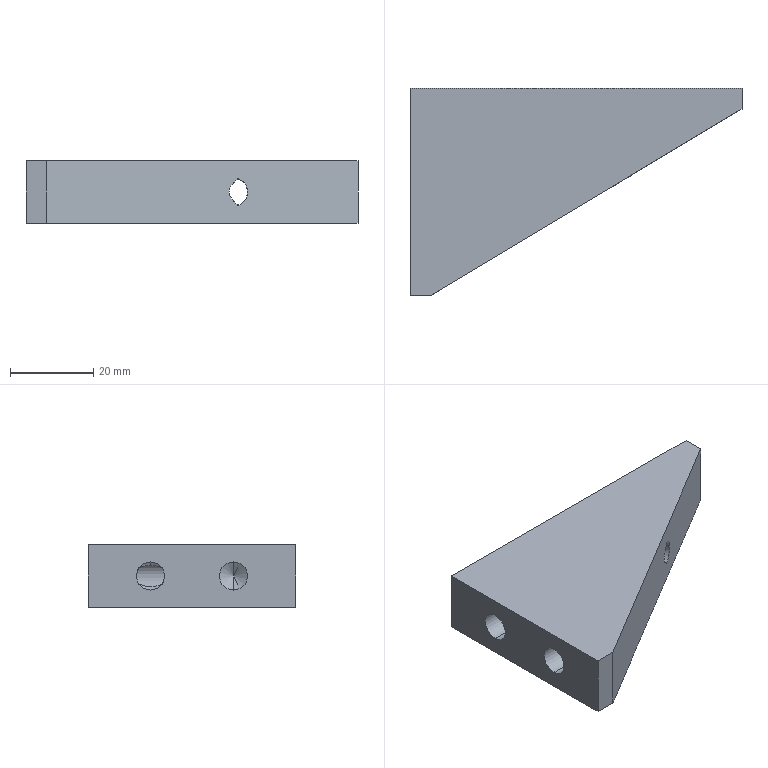Part | SolidWorks | features HoleWzd 2, Extrusion 1 | 1 solid | 25 faces | box 80 x 50 x 15 mm | volume 31407 mm3 | cone 10 | cylinder 8 | plane 7 | commonest cylinder face diameters 6.8 x8
STEP:
#1=CARTESIAN_POINT('',(22.757,35.,10.056));
#2=VERTEX_POINT('',#1);
#3=CARTESIAN_POINT('',(22.25,37.75,9.499));
#4=VERTEX_POINT('',#3);
#5=CARTESIAN_POINT('',(22.757,35.,10.056));
#6=CARTESIAN_POINT('',(22.757,35.242,10.056));
#7=CARTESIAN_POINT('',(22.744,35.483,10.044));
#8=CARTESIAN_POINT('',(22.692,35.956,9.997));
#9=CARTESIAN_POINT('',(22.655,36.19,9.963));
#10=CARTESIAN_POINT('',(22.562,36.651,9.871));
#11=CARTESIAN_POINT('',(22.506,36.88,9.813));
#12=CARTESIAN_POINT('',(22.384,37.325,9.674));
#13=CARTESIAN_POINT('',(22.318,37.541,9.594));
#14=CARTESIAN_POINT('',(22.25,37.75,9.499));
#15=B_SPLINE_CURVE_WITH_KNOTS('',3,(#5,#6,#7,#8,#9,#10,#11,#12,#13,#14),.UNSPECIFIED.,.F.,.F.,(4,2,2,2,4),(0.003573,0.004291,0.005009,0.005727,0.006445),.UNSPECIFIED.);
#16=EDGE_CURVE('',#2,#4,#15,.T.);
#17=ORIENTED_EDGE('',*,*,#16,.F.);
#18=CARTESIAN_POINT('',(22.25,35.,10.9));
#19=VERTEX_POINT('',#18);
#20=CARTESIAN_POINT('',(22.25,35.,10.9));
#21=DIRECTION('',(-0.515,0.,0.8572));
#22=VECTOR('',#21,1000.);
#23=LINE('',#20,#22);
#24=EDGE_CURVE('',#2,#19,#23,.T.);
#25=ORIENTED_EDGE('',*,*,#24,.T.);
#26=CARTESIAN_POINT('',(22.25,35.,7.5));
#27=DIRECTION('',(-1.,0.,0.));
#28=DIRECTION('',(0.,0.,1.));
#29=AXIS2_PLACEMENT_3D('',#26,#27,#28);
#30=CIRCLE('',#29,3.4);
#31=EDGE_CURVE('',#19,#4,#30,.T.);
#32=ORIENTED_EDGE('',*,*,#31,.T.);
#33=EDGE_LOOP('',(#17,#25,#32));
#34=FACE_OUTER_BOUND('',#33,.T.);
#35=CARTESIAN_POINT('',(22.25,35.,7.5));
#36=DIRECTION('',(-1.,0.,0.));
#37=DIRECTION('',(0.,0.,1.));
#38=AXIS2_PLACEMENT_3D('',#35,#36,#37);
#39=CONICAL_SURFACE('',#38,3.4,1.03);
#40=ADVANCED_FACE('',(#34),#39,.F.);
#41=CARTESIAN_POINT('',(22.25,35.,4.1));
#42=VERTEX_POINT('',#41);
#43=CARTESIAN_POINT('',(22.25,32.25,5.501));
#44=VERTEX_POINT('',#43);
#45=CARTESIAN_POINT('',(22.25,35.,7.5));
#46=DIRECTION('',(-1.,0.,0.));
#47=DIRECTION('',(0.,0.,1.));
#48=AXIS2_PLACEMENT_3D('',#45,#46,#47);
#49=CIRCLE('',#48,3.4);
#50=EDGE_CURVE('',#42,#44,#49,.T.);
#51=ORIENTED_EDGE('',*,*,#50,.F.);
#52=CARTESIAN_POINT('',(0.,35.,4.1));
#53=VERTEX_POINT('',#52);
#54=CARTESIAN_POINT('',(0.,35.,4.1));
#55=DIRECTION('',(-1.,0.,0.));
#56=VECTOR('',#55,1000.);
#57=LINE('',#54,#56);
#58=EDGE_CURVE('',#42,#53,#57,.T.);
#59=ORIENTED_EDGE('',*,*,#58,.T.);
#60=CARTESIAN_POINT('',(0.,35.,10.9));
#61=VERTEX_POINT('',#60);
#62=CARTESIAN_POINT('',(0.,35.,7.5));
#63=DIRECTION('',(-1.,0.,0.));
#64=DIRECTION('',(0.,0.,1.));
#65=AXIS2_PLACEMENT_3D('',#62,#63,#64);
#66=CIRCLE('',#65,3.4);
#67=EDGE_CURVE('',#53,#61,#66,.T.);
#68=ORIENTED_EDGE('',*,*,#67,.T.);
#69=CARTESIAN_POINT('',(0.,35.,10.9));
#70=DIRECTION('',(-1.,0.,0.));
#71=VECTOR('',#70,1000.);
#72=LINE('',#69,#71);
#73=EDGE_CURVE('',#19,#61,#72,.T.);
#74=ORIENTED_EDGE('',*,*,#73,.F.);
#75=CARTESIAN_POINT('',(22.25,32.25,9.499));
#76=VERTEX_POINT('',#75);
#77=CARTESIAN_POINT('',(22.25,35.,7.5));
#78=DIRECTION('',(-1.,0.,0.));
#79=DIRECTION('',(0.,0.,1.));
#80=AXIS2_PLACEMENT_3D('',#77,#78,#79);
#81=CIRCLE('',#80,3.4);
#82=EDGE_CURVE('',#76,#19,#81,.T.);
#83=ORIENTED_EDGE('',*,*,#82,.F.);
#84=CARTESIAN_POINT('',(22.25,32.25,5.501));
#85=CARTESIAN_POINT('',(21.352,31.352,6.736));
#86=CARTESIAN_POINT('',(21.352,31.352,8.264));
#87=CARTESIAN_POINT('',(22.25,32.25,9.499));
#88=(BOUNDED_CURVE()B_SPLINE_CURVE(3,(#84,#85,#86,#87),.UNSPECIFIED.,.F.,.F.)B_SPLINE_CURVE_WITH_KNOTS((4,4),(2.513,3.77),.UNSPECIFIED.)CURVE()GEOMETRIC_REPRESENTATION_ITEM()RATIONAL_B_SPLINE_CURVE((1.,0.8725,0.8725,1.))REPRESENTATION_ITEM(''));
#89=EDGE_CURVE('',#44,#76,#88,.T.);
#90=ORIENTED_EDGE('',*,*,#89,.F.);
#91=EDGE_LOOP('',(#51,#59,#68,#74,#83,#90));
#92=FACE_OUTER_BOUND('',#91,.T.);
#93=CARTESIAN_POINT('',(0.,35.,7.5));
#94=DIRECTION('',(-1.,0.,0.));
#95=DIRECTION('',(0.,0.,1.));
#96=AXIS2_PLACEMENT_3D('',#93,#94,#95);
#97=CYLINDRICAL_SURFACE('',#96,3.4);
#98=ADVANCED_FACE('',(#92),#97,.F.);
#99=CARTESIAN_POINT('',(22.25,15.,4.1));
#100=VERTEX_POINT('',#99);
#101=CARTESIAN_POINT('',(22.25,15.,10.9));
#102=VERTEX_POINT('',#101);
#103=CARTESIAN_POINT('',(22.25,15.,7.5));
#104=DIRECTION('',(-1.,0.,0.));
#105=DIRECTION('',(0.,0.,1.));
#106=AXIS2_PLACEMENT_3D('',#103,#104,#105);
#107=CIRCLE('',#106,3.4);
#108=EDGE_CURVE('',#100,#102,#107,.T.);
#109=ORIENTED_EDGE('',*,*,#108,.F.);
#110=CARTESIAN_POINT('',(0.,15.,4.1));
#111=VERTEX_POINT('',#110);
#112=CARTESIAN_POINT('',(0.,15.,4.1));
#113=DIRECTION('',(-1.,0.,0.));
#114=VECTOR('',#113,1000.);
#115=LINE('',#112,#114);
#116=EDGE_CURVE('',#100,#111,#115,.T.);
#117=ORIENTED_EDGE('',*,*,#116,.T.);
#118=CARTESIAN_POINT('',(0.,15.,10.9));
#119=VERTEX_POINT('',#118);
#120=CARTESIAN_POINT('',(0.,15.,7.5));
#121=DIRECTION('',(-1.,0.,0.));
#122=DIRECTION('',(0.,0.,1.));
#123=AXIS2_PLACEMENT_3D('',#120,#121,#122);
#124=CIRCLE('',#123,3.4);
#125=EDGE_CURVE('',#111,#119,#124,.T.);
#126=ORIENTED_EDGE('',*,*,#125,.T.);
#127=CARTESIAN_POINT('',(0.,15.,10.9));
#128=DIRECTION('',(-1.,0.,0.));
#129=VECTOR('',#128,1000.);
#130=LINE('',#127,#129);
#131=EDGE_CURVE('',#102,#119,#130,.T.);
#132=ORIENTED_EDGE('',*,*,#131,.F.);
#133=EDGE_LOOP('',(#109,#117,#126,#132));
#134=FACE_OUTER_BOUND('',#133,.T.);
#135=CARTESIAN_POINT('',(0.,15.,7.5));
#136=DIRECTION('',(-1.,0.,0.));
#137=DIRECTION('',(0.,0.,1.));
#138=AXIS2_PLACEMENT_3D('',#135,#136,#137);
#139=CYLINDRICAL_SURFACE('',#138,3.4);
#140=ADVANCED_FACE('',(#134),#139,.F.);
#141=CARTESIAN_POINT('',(24.293,15.,7.5));
#142=VERTEX_POINT('',#141);
#143=CARTESIAN_POINT('',(22.25,15.,10.9));
#144=DIRECTION('',(-0.515,0.,0.8572));
#145=VECTOR('',#144,1000.);
#146=LINE('',#143,#145);
#147=EDGE_CURVE('',#142,#102,#146,.T.);
#148=ORIENTED_EDGE('',*,*,#147,.F.);
#149=CARTESIAN_POINT('',(22.25,15.,4.1));
#150=DIRECTION('',(-0.515,0.,-0.8572));
#151=VECTOR('',#150,1000.);
#152=LINE('',#149,#151);
#153=EDGE_CURVE('',#142,#100,#152,.T.);
#154=ORIENTED_EDGE('',*,*,#153,.T.);
#155=ORIENTED_EDGE('',*,*,#108,.T.);
#156=EDGE_LOOP('',(#148,#154,#155));
#157=FACE_OUTER_BOUND('',#156,.T.);
#158=CARTESIAN_POINT('',(22.25,15.,7.5));
#159=DIRECTION('',(-1.,0.,0.));
#160=DIRECTION('',(0.,0.,1.));
#161=AXIS2_PLACEMENT_3D('',#158,#159,#160);
#162=CONICAL_SURFACE('',#161,3.4,1.03);
#163=ADVANCED_FACE('',(#157),#162,.F.);
#164=CARTESIAN_POINT('',(22.25,37.75,5.501));
#165=VERTEX_POINT('',#164);
#166=CARTESIAN_POINT('',(22.25,37.75,9.499));
#167=CARTESIAN_POINT('',(21.352,38.648,8.264));
#168=CARTESIAN_POINT('',(21.352,38.648,6.736));
#169=CARTESIAN_POINT('',(22.25,37.75,5.501));
#170=(BOUNDED_CURVE()B_SPLINE_CURVE(3,(#166,#167,#168,#169),.UNSPECIFIED.,.F.,.F.)B_SPLINE_CURVE_WITH_KNOTS((4,4),(5.655,6.912),.UNSPECIFIED.)CURVE()GEOMETRIC_REPRESENTATION_ITEM()RATIONAL_B_SPLINE_CURVE((1.,0.8725,0.8725,1.))REPRESENTATION_ITEM(''));
#171=EDGE_CURVE('',#4,#165,#170,.T.);
#172=ORIENTED_EDGE('',*,*,#171,.T.);
#173=CARTESIAN_POINT('',(22.25,37.75,5.501));
#174=CARTESIAN_POINT('',(22.318,37.541,5.406));
#175=CARTESIAN_POINT('',(22.384,37.325,5.326));
#176=CARTESIAN_POINT('',(22.506,36.881,5.187));
#177=CARTESIAN_POINT('',(22.562,36.651,5.129));
#178=CARTESIAN_POINT('',(22.702,35.958,4.991));
#179=CARTESIAN_POINT('',(22.757,35.486,4.945));
#180=CARTESIAN_POINT('',(22.757,34.76,4.944));
#181=CARTESIAN_POINT('',(22.744,34.519,4.956));
#182=CARTESIAN_POINT('',(22.693,34.045,5.003));
#183=CARTESIAN_POINT('',(22.655,33.812,5.037));
#184=CARTESIAN_POINT('',(22.562,33.35,5.129));
#185=CARTESIAN_POINT('',(22.506,33.12,5.187));
#186=CARTESIAN_POINT('',(22.385,32.676,5.326));
#187=CARTESIAN_POINT('',(22.319,32.46,5.406));
#188=CARTESIAN_POINT('',(22.25,32.25,5.501));
#189=B_SPLINE_CURVE_WITH_KNOTS('',3,(#173,#174,#175,#176,#177,#178,#179,#180,#181,#182,#183,#184,#185,#186,#187,#188),.UNSPECIFIED.,.F.,.F.,(4,2,2,2,2,2,2,4),(0.0006976,0.001416,0.002134,0.003571,0.004289,0.005008,0.005726,0.006445),.UNSPECIFIED.);
#190=EDGE_CURVE('',#165,#44,#189,.T.);
#191=ORIENTED_EDGE('',*,*,#190,.T.);
#192=ORIENTED_EDGE('',*,*,#89,.T.);
#193=CARTESIAN_POINT('',(22.25,32.25,9.499));
#194=CARTESIAN_POINT('',(22.319,32.46,9.594));
#195=CARTESIAN_POINT('',(22.385,32.675,9.674));
#196=CARTESIAN_POINT('',(22.506,33.12,9.813));
#197=CARTESIAN_POINT('',(22.562,33.35,9.871));
#198=CARTESIAN_POINT('',(22.702,34.043,10.009));
#199=CARTESIAN_POINT('',(22.757,34.515,10.056));
#200=CARTESIAN_POINT('',(22.757,35.,10.056));
#201=B_SPLINE_CURVE_WITH_KNOTS('',3,(#193,#194,#195,#196,#197,#198,#199,#200),.UNSPECIFIED.,.F.,.F.,(4,2,2,4),(0.0006976,0.001416,0.002135,0.003573),.UNSPECIFIED.);
#202=EDGE_CURVE('',#76,#2,#201,.T.);
#203=ORIENTED_EDGE('',*,*,#202,.T.);
#204=ORIENTED_EDGE('',*,*,#16,.T.);
#205=EDGE_LOOP('',(#172,#191,#192,#203,#204));
#206=FACE_BOUND('',#205,.T.);
#207=CARTESIAN_POINT('',(25.,27.75,4.1));
#208=VERTEX_POINT('',#207);
#209=CARTESIAN_POINT('',(25.,27.75,10.9));
#210=VERTEX_POINT('',#209);
#211=CARTESIAN_POINT('',(25.,27.75,7.5));
#212=DIRECTION('',(0.,1.,0.));
#213=DIRECTION('',(0.,0.,1.));
#214=AXIS2_PLACEMENT_3D('',#211,#212,#213);
#215=CIRCLE('',#214,3.4);
#216=EDGE_CURVE('',#208,#210,#215,.T.);
#217=ORIENTED_EDGE('',*,*,#216,.F.);
#218=CARTESIAN_POINT('',(25.,50.,4.1));
#219=VERTEX_POINT('',#218);
#220=CARTESIAN_POINT('',(25.,50.,4.1));
#221=DIRECTION('',(0.,1.,0.));
#222=VECTOR('',#221,1000.);
#223=LINE('',#220,#222);
#224=EDGE_CURVE('',#208,#219,#223,.T.);
#225=ORIENTED_EDGE('',*,*,#224,.T.);
#226=CARTESIAN_POINT('',(25.,50.,10.9));
#227=VERTEX_POINT('',#226);
#228=CARTESIAN_POINT('',(25.,50.,7.5));
#229=DIRECTION('',(0.,1.,0.));
#230=DIRECTION('',(0.,0.,1.));
#231=AXIS2_PLACEMENT_3D('',#228,#229,#230);
#232=CIRCLE('',#231,3.4);
#233=EDGE_CURVE('',#219,#227,#232,.T.);
#234=ORIENTED_EDGE('',*,*,#233,.T.);
#235=CARTESIAN_POINT('',(25.,50.,10.9));
#236=DIRECTION('',(0.,1.,0.));
#237=VECTOR('',#236,1000.);
#238=LINE('',#235,#237);
#239=EDGE_CURVE('',#210,#227,#238,.T.);
#240=ORIENTED_EDGE('',*,*,#239,.F.);
#241=EDGE_LOOP('',(#217,#225,#234,#240));
#242=FACE_OUTER_BOUND('',#241,.T.);
#243=CARTESIAN_POINT('',(25.,50.,7.5));
#244=DIRECTION('',(0.,1.,0.));
#245=DIRECTION('',(0.,0.,1.));
#246=AXIS2_PLACEMENT_3D('',#243,#244,#245);
#247=CYLINDRICAL_SURFACE('',#246,3.4);
#248=ADVANCED_FACE('',(#206,#242),#247,.F.);
#249=CARTESIAN_POINT('',(25.,25.707,7.5));
#250=VERTEX_POINT('',#249);
#251=CARTESIAN_POINT('',(25.,27.75,10.9));
#252=DIRECTION('',(0.,0.515,0.8572));
#253=VECTOR('',#252,1000.);
#254=LINE('',#251,#253);
#255=EDGE_CURVE('',#250,#210,#254,.T.);
#256=ORIENTED_EDGE('',*,*,#255,.F.);
#257=CARTESIAN_POINT('',(25.,27.75,4.1));
#258=DIRECTION('',(0.,0.515,-0.8572));
#259=VECTOR('',#258,1000.);
#260=LINE('',#257,#259);
#261=EDGE_CURVE('',#250,#208,#260,.T.);
#262=ORIENTED_EDGE('',*,*,#261,.T.);
#263=ORIENTED_EDGE('',*,*,#216,.T.);
#264=EDGE_LOOP('',(#256,#262,#263));
#265=FACE_OUTER_BOUND('',#264,.T.);
#266=CARTESIAN_POINT('',(25.,27.75,7.5));
#267=DIRECTION('',(0.,1.,0.));
#268=DIRECTION('',(0.,0.,1.));
#269=AXIS2_PLACEMENT_3D('',#266,#267,#268);
#270=CONICAL_SURFACE('',#269,3.4,1.03);
#271=ADVANCED_FACE('',(#265),#270,.F.);
#272=CARTESIAN_POINT('',(50.,27.,5.348));
#273=VERTEX_POINT('',#272);
#274=CARTESIAN_POINT('',(50.,27.,9.652));
#275=VERTEX_POINT('',#274);
#276=CARTESIAN_POINT('',(50.,27.,5.348));
#277=CARTESIAN_POINT('',(48.564,26.138,6.782));
#278=CARTESIAN_POINT('',(48.564,26.138,8.218));
#279=CARTESIAN_POINT('',(50.,27.,9.652));
#280=(BOUNDED_CURVE()B_SPLINE_CURVE(3,(#276,#277,#278,#279),.UNSPECIFIED.,.F.,.F.)B_SPLINE_CURVE_WITH_KNOTS((4,4),(3.088,3.195),.UNSPECIFIED.)CURVE()GEOMETRIC_REPRESENTATION_ITEM()RATIONAL_B_SPLINE_CURVE((1.,0.999,0.999,1.))REPRESENTATION_ITEM(''));
#281=EDGE_CURVE('',#273,#275,#280,.T.);
#282=ORIENTED_EDGE('',*,*,#281,.F.);
#283=CARTESIAN_POINT('',(50.,27.75,4.1));
#284=VERTEX_POINT('',#283);
#285=CARTESIAN_POINT('',(50.,27.75,4.1));
#286=DIRECTION('',(0.,0.515,-0.8572));
#287=VECTOR('',#286,1000.);
#288=LINE('',#285,#287);
#289=EDGE_CURVE('',#273,#284,#288,.T.);
#290=ORIENTED_EDGE('',*,*,#289,.T.);
#291=CARTESIAN_POINT('',(50.,27.75,10.9));
#292=VERTEX_POINT('',#291);
#293=CARTESIAN_POINT('',(50.,27.75,7.5));
#294=DIRECTION('',(0.,1.,0.));
#295=DIRECTION('',(0.,0.,1.));
#296=AXIS2_PLACEMENT_3D('',#293,#294,#295);
#297=CIRCLE('',#296,3.4);
#298=EDGE_CURVE('',#284,#292,#297,.T.);
#299=ORIENTED_EDGE('',*,*,#298,.T.);
#300=CARTESIAN_POINT('',(50.,27.75,10.9));
#301=DIRECTION('',(0.,0.515,0.8572));
#302=VECTOR('',#301,1000.);
#303=LINE('',#300,#302);
#304=EDGE_CURVE('',#275,#292,#303,.T.);
#305=ORIENTED_EDGE('',*,*,#304,.F.);
#306=EDGE_LOOP('',(#282,#290,#299,#305));
#307=FACE_OUTER_BOUND('',#306,.T.);
#308=CARTESIAN_POINT('',(50.,27.75,7.5));
#309=DIRECTION('',(0.,1.,0.));
#310=DIRECTION('',(0.,0.,1.));
#311=AXIS2_PLACEMENT_3D('',#308,#309,#310);
#312=CONICAL_SURFACE('',#311,3.4,1.03);
#313=ADVANCED_FACE('',(#307),#312,.F.);
#314=CARTESIAN_POINT('',(51.25,27.75,10.662));
#315=VERTEX_POINT('',#314);
#316=CARTESIAN_POINT('',(50.,27.,9.652));
#317=CARTESIAN_POINT('',(50.337,27.202,9.989));
#318=CARTESIAN_POINT('',(50.754,27.452,10.325));
#319=CARTESIAN_POINT('',(51.25,27.75,10.662));
#320=(BOUNDED_CURVE()B_SPLINE_CURVE(3,(#316,#317,#318,#319),.UNSPECIFIED.,.F.,.F.)B_SPLINE_CURVE_WITH_KNOTS((4,4),(3.195,3.22),.UNSPECIFIED.)CURVE()GEOMETRIC_REPRESENTATION_ITEM()RATIONAL_B_SPLINE_CURVE((1.,0.9999,0.9999,1.))REPRESENTATION_ITEM(''));
#321=EDGE_CURVE('',#275,#315,#320,.T.);
#322=ORIENTED_EDGE('',*,*,#321,.F.);
#323=ORIENTED_EDGE('',*,*,#304,.T.);
#324=CARTESIAN_POINT('',(50.,27.75,7.5));
#325=DIRECTION('',(0.,1.,0.));
#326=DIRECTION('',(0.,0.,1.));
#327=AXIS2_PLACEMENT_3D('',#324,#325,#326);
#328=CIRCLE('',#327,3.4);
#329=EDGE_CURVE('',#292,#315,#328,.T.);
#330=ORIENTED_EDGE('',*,*,#329,.T.);
#331=EDGE_LOOP('',(#322,#323,#330));
#332=FACE_OUTER_BOUND('',#331,.T.);
#333=CARTESIAN_POINT('',(50.,27.75,7.5));
#334=DIRECTION('',(0.,1.,0.));
#335=DIRECTION('',(0.,0.,1.));
#336=AXIS2_PLACEMENT_3D('',#333,#334,#335);
#337=CONICAL_SURFACE('',#336,3.4,1.03);
#338=ADVANCED_FACE('',(#332),#337,.F.);
#339=ORIENTED_EDGE('',*,*,#298,.F.);
#340=CARTESIAN_POINT('',(50.,50.,4.1));
#341=VERTEX_POINT('',#340);
#342=CARTESIAN_POINT('',(50.,50.,4.1));
#343=DIRECTION('',(0.,1.,0.));
#344=VECTOR('',#343,1000.);
#345=LINE('',#342,#344);
#346=EDGE_CURVE('',#284,#341,#345,.T.);
#347=ORIENTED_EDGE('',*,*,#346,.T.);
#348=CARTESIAN_POINT('',(50.,50.,10.9));
#349=VERTEX_POINT('',#348);
#350=CARTESIAN_POINT('',(50.,50.,7.5));
#351=DIRECTION('',(0.,1.,0.));
#352=DIRECTION('',(0.,0.,1.));
#353=AXIS2_PLACEMENT_3D('',#350,#351,#352);
#354=CIRCLE('',#353,3.4);
#355=EDGE_CURVE('',#341,#349,#354,.T.);
#356=ORIENTED_EDGE('',*,*,#355,.T.);
#357=CARTESIAN_POINT('',(50.,50.,10.9));
#358=DIRECTION('',(0.,1.,0.));
#359=VECTOR('',#358,1000.);
#360=LINE('',#357,#359);
#361=EDGE_CURVE('',#292,#349,#360,.T.);
#362=ORIENTED_EDGE('',*,*,#361,.F.);
#363=EDGE_LOOP('',(#339,#347,#356,#362));
#364=FACE_OUTER_BOUND('',#363,.T.);
#365=CARTESIAN_POINT('',(50.,50.,7.5));
#366=DIRECTION('',(0.,1.,0.));
#367=DIRECTION('',(0.,0.,1.));
#368=AXIS2_PLACEMENT_3D('',#365,#366,#367);
#369=CYLINDRICAL_SURFACE('',#368,3.4);
#370=ADVANCED_FACE('',(#364),#369,.F.);
#371=CARTESIAN_POINT('',(0.,0.,0.));
#372=VERTEX_POINT('',#371);
#373=CARTESIAN_POINT('',(5.,0.,0.));
#374=VERTEX_POINT('',#373);
#375=CARTESIAN_POINT('',(5.,0.,0.));
#376=DIRECTION('',(1.,0.,0.));
#377=VECTOR('',#376,1000.);
#378=LINE('',#375,#377);
#379=EDGE_CURVE('',#372,#374,#378,.T.);
#380=ORIENTED_EDGE('',*,*,#379,.T.);
#381=CARTESIAN_POINT('',(5.,0.,15.));
#382=VERTEX_POINT('',#381);
#383=CARTESIAN_POINT('',(5.,0.,15.));
#384=DIRECTION('',(0.,0.,-1.));
#385=VECTOR('',#384,1000.);
#386=LINE('',#383,#385);
#387=EDGE_CURVE('',#382,#374,#386,.T.);
#388=ORIENTED_EDGE('',*,*,#387,.F.);
#389=CARTESIAN_POINT('',(0.,0.,15.));
#390=VERTEX_POINT('',#389);
#391=CARTESIAN_POINT('',(5.,0.,15.));
#392=DIRECTION('',(1.,0.,0.));
#393=VECTOR('',#392,1000.);
#394=LINE('',#391,#393);
#395=EDGE_CURVE('',#390,#382,#394,.T.);
#396=ORIENTED_EDGE('',*,*,#395,.F.);
#397=CARTESIAN_POINT('',(0.,0.,15.));
#398=DIRECTION('',(0.,0.,-1.));
#399=VECTOR('',#398,1000.);
#400=LINE('',#397,#399);
#401=EDGE_CURVE('',#390,#372,#400,.T.);
#402=ORIENTED_EDGE('',*,*,#401,.T.);
#403=EDGE_LOOP('',(#380,#388,#396,#402));
#404=FACE_OUTER_BOUND('',#403,.T.);
#405=CARTESIAN_POINT('',(5.,0.,15.));
#406=DIRECTION('',(0.,1.,0.));
#407=DIRECTION('',(-1.,0.,0.));
#408=AXIS2_PLACEMENT_3D('',#405,#406,#407);
#409=PLANE('',#408);
#410=ADVANCED_FACE('',(#404),#409,.F.);
#411=CARTESIAN_POINT('',(51.25,27.75,4.338));
#412=VERTEX_POINT('',#411);
#413=CARTESIAN_POINT('',(51.25,27.75,4.338));
#414=CARTESIAN_POINT('',(50.754,27.452,4.675));
#415=CARTESIAN_POINT('',(50.337,27.202,5.011));
#416=CARTESIAN_POINT('',(50.,27.,5.348));
#417=(BOUNDED_CURVE()B_SPLINE_CURVE(3,(#413,#414,#415,#416),.UNSPECIFIED.,.F.,.F.)B_SPLINE_CURVE_WITH_KNOTS((4,4),(3.063,3.088),.UNSPECIFIED.)CURVE()GEOMETRIC_REPRESENTATION_ITEM()RATIONAL_B_SPLINE_CURVE((1.,0.9999,0.9999,1.))REPRESENTATION_ITEM(''));
#418=EDGE_CURVE('',#412,#273,#417,.T.);
#419=ORIENTED_EDGE('',*,*,#418,.T.);
#420=ORIENTED_EDGE('',*,*,#281,.T.);
#421=ORIENTED_EDGE('',*,*,#321,.T.);
#422=CARTESIAN_POINT('',(51.25,27.75,10.662));
#423=CARTESIAN_POINT('',(54.639,29.783,9.322));
#424=CARTESIAN_POINT('',(54.639,29.783,5.678));
#425=CARTESIAN_POINT('',(51.25,27.75,4.338));
#426=(BOUNDED_CURVE()B_SPLINE_CURVE(3,(#422,#423,#424,#425),.UNSPECIFIED.,.F.,.T.)B_SPLINE_CURVE_WITH_KNOTS((4,4),(5.089,7.478),.UNSPECIFIED.)CURVE()GEOMETRIC_REPRESENTATION_ITEM()RATIONAL_B_SPLINE_CURVE((1.,0.5784,0.5784,1.))REPRESENTATION_ITEM(''));
#427=EDGE_CURVE('',#315,#412,#426,.T.);
#428=ORIENTED_EDGE('',*,*,#427,.T.);
#429=EDGE_LOOP('',(#419,#420,#421,#428));
#430=FACE_BOUND('',#429,.T.);
#431=CARTESIAN_POINT('',(80.,45.,0.));
#432=VERTEX_POINT('',#431);
#433=CARTESIAN_POINT('',(80.,45.,0.));
#434=DIRECTION('',(0.8575,0.5145,0.));
#435=VECTOR('',#434,1000.);
#436=LINE('',#433,#435);
#437=EDGE_CURVE('',#374,#432,#436,.T.);
#438=ORIENTED_EDGE('',*,*,#437,.T.);
#439=CARTESIAN_POINT('',(80.,45.,15.));
#440=VERTEX_POINT('',#439);
#441=CARTESIAN_POINT('',(80.,45.,15.));
#442=DIRECTION('',(0.,0.,-1.));
#443=VECTOR('',#442,1000.);
#444=LINE('',#441,#443);
#445=EDGE_CURVE('',#440,#432,#444,.T.);
#446=ORIENTED_EDGE('',*,*,#445,.F.);
#447=CARTESIAN_POINT('',(80.,45.,15.));
#448=DIRECTION('',(0.8575,0.5145,0.));
#449=VECTOR('',#448,1000.);
#450=LINE('',#447,#449);
#451=EDGE_CURVE('',#382,#440,#450,.T.);
#452=ORIENTED_EDGE('',*,*,#451,.F.);
#453=ORIENTED_EDGE('',*,*,#387,.T.);
#454=EDGE_LOOP('',(#438,#446,#452,#453));
#455=FACE_OUTER_BOUND('',#454,.T.);
#456=CARTESIAN_POINT('',(80.,45.,15.));
#457=DIRECTION('',(-0.5145,0.8575,0.));
#458=DIRECTION('',(-0.8575,-0.5145,0.));
#459=AXIS2_PLACEMENT_3D('',#456,#457,#458);
#460=PLANE('',#459);
#461=ADVANCED_FACE('',(#430,#455),#460,.F.);
#462=CARTESIAN_POINT('',(80.,50.,0.));
#463=VERTEX_POINT('',#462);
#464=CARTESIAN_POINT('',(80.,50.,0.));
#465=DIRECTION('',(0.,1.,0.));
#466=VECTOR('',#465,1000.);
#467=LINE('',#464,#466);
#468=EDGE_CURVE('',#432,#463,#467,.T.);
#469=ORIENTED_EDGE('',*,*,#468,.T.);
#470=CARTESIAN_POINT('',(80.,50.,15.));
#471=VERTEX_POINT('',#470);
#472=CARTESIAN_POINT('',(80.,50.,15.));
#473=DIRECTION('',(0.,0.,-1.));
#474=VECTOR('',#473,1000.);
#475=LINE('',#472,#474);
#476=EDGE_CURVE('',#471,#463,#475,.T.);
#477=ORIENTED_EDGE('',*,*,#476,.F.);
#478=CARTESIAN_POINT('',(80.,50.,15.));
#479=DIRECTION('',(0.,1.,0.));
#480=VECTOR('',#479,1000.);
#481=LINE('',#478,#480);
#482=EDGE_CURVE('',#440,#471,#481,.T.);
#483=ORIENTED_EDGE('',*,*,#482,.F.);
#484=ORIENTED_EDGE('',*,*,#445,.T.);
#485=EDGE_LOOP('',(#469,#477,#483,#484));
#486=FACE_OUTER_BOUND('',#485,.T.);
#487=CARTESIAN_POINT('',(80.,50.,15.));
#488=DIRECTION('',(-1.,0.,0.));
#489=DIRECTION('',(0.,0.,1.));
#490=AXIS2_PLACEMENT_3D('',#487,#488,#489);
#491=PLANE('',#490);
#492=ADVANCED_FACE('',(#486),#491,.F.);
#493=CARTESIAN_POINT('',(25.,50.,7.5));
#494=DIRECTION('',(0.,1.,0.));
#495=DIRECTION('',(0.,0.,1.));
#496=AXIS2_PLACEMENT_3D('',#493,#494,#495);
#497=CIRCLE('',#496,3.4);
#498=EDGE_CURVE('',#227,#219,#497,.T.);
#499=ORIENTED_EDGE('',*,*,#498,.F.);
#500=ORIENTED_EDGE('',*,*,#233,.F.);
#501=EDGE_LOOP('',(#499,#500));
#502=FACE_BOUND('',#501,.T.);
#503=CARTESIAN_POINT('',(50.,50.,7.5));
#504=DIRECTION('',(0.,1.,0.));
#505=DIRECTION('',(0.,0.,1.));
#506=AXIS2_PLACEMENT_3D('',#503,#504,#505);
#507=CIRCLE('',#506,3.4);
#508=EDGE_CURVE('',#349,#341,#507,.T.);
#509=ORIENTED_EDGE('',*,*,#508,.F.);
#510=ORIENTED_EDGE('',*,*,#355,.F.);
#511=EDGE_LOOP('',(#509,#510));
#512=FACE_BOUND('',#511,.T.);
#513=CARTESIAN_POINT('',(0.,50.,0.));
#514=VERTEX_POINT('',#513);
#515=CARTESIAN_POINT('',(0.,50.,0.));
#516=DIRECTION('',(-1.,0.,0.));
#517=VECTOR('',#516,1000.);
#518=LINE('',#515,#517);
#519=EDGE_CURVE('',#463,#514,#518,.T.);
#520=ORIENTED_EDGE('',*,*,#519,.T.);
#521=CARTESIAN_POINT('',(0.,50.,15.));
#522=VERTEX_POINT('',#521);
#523=CARTESIAN_POINT('',(0.,50.,15.));
#524=DIRECTION('',(0.,0.,-1.));
#525=VECTOR('',#524,1000.);
#526=LINE('',#523,#525);
#527=EDGE_CURVE('',#522,#514,#526,.T.);
#528=ORIENTED_EDGE('',*,*,#527,.F.);
#529=CARTESIAN_POINT('',(0.,50.,15.));
#530=DIRECTION('',(-1.,0.,0.));
#531=VECTOR('',#530,1000.);
#532=LINE('',#529,#531);
#533=EDGE_CURVE('',#471,#522,#532,.T.);
#534=ORIENTED_EDGE('',*,*,#533,.F.);
#535=ORIENTED_EDGE('',*,*,#476,.T.);
#536=EDGE_LOOP('',(#520,#528,#534,#535));
#537=FACE_OUTER_BOUND('',#536,.T.);
#538=CARTESIAN_POINT('',(0.,50.,15.));
#539=DIRECTION('',(0.,-1.,0.));
#540=DIRECTION('',(0.,0.,-1.));
#541=AXIS2_PLACEMENT_3D('',#538,#539,#540);
#542=PLANE('',#541);
#543=ADVANCED_FACE('',(#502,#512,#537),#542,.F.);
#544=CARTESIAN_POINT('',(0.,35.,7.5));
#545=DIRECTION('',(-1.,0.,0.));
#546=DIRECTION('',(0.,0.,1.));
#547=AXIS2_PLACEMENT_3D('',#544,#545,#546);
#548=CIRCLE('',#547,3.4);
#549=EDGE_CURVE('',#61,#53,#548,.T.);
#550=ORIENTED_EDGE('',*,*,#549,.F.);
#551=ORIENTED_EDGE('',*,*,#67,.F.);
#552=EDGE_LOOP('',(#550,#551));
#553=FACE_BOUND('',#552,.T.);
#554=CARTESIAN_POINT('',(0.,15.,7.5));
#555=DIRECTION('',(-1.,0.,0.));
#556=DIRECTION('',(0.,0.,1.));
#557=AXIS2_PLACEMENT_3D('',#554,#555,#556);
#558=CIRCLE('',#557,3.4);
#559=EDGE_CURVE('',#119,#111,#558,.T.);
#560=ORIENTED_EDGE('',*,*,#559,.F.);
#561=ORIENTED_EDGE('',*,*,#125,.F.);
#562=EDGE_LOOP('',(#560,#561));
#563=FACE_BOUND('',#562,.T.);
#564=CARTESIAN_POINT('',(0.,0.,0.));
#565=DIRECTION('',(0.,-1.,0.));
#566=VECTOR('',#565,1000.);
#567=LINE('',#564,#566);
#568=EDGE_CURVE('',#514,#372,#567,.T.);
#569=ORIENTED_EDGE('',*,*,#568,.T.);
#570=ORIENTED_EDGE('',*,*,#401,.F.);
#571=CARTESIAN_POINT('',(0.,0.,15.));
#572=DIRECTION('',(0.,-1.,0.));
#573=VECTOR('',#572,1000.);
#574=LINE('',#571,#573);
#575=EDGE_CURVE('',#522,#390,#574,.T.);
#576=ORIENTED_EDGE('',*,*,#575,.F.);
#577=ORIENTED_EDGE('',*,*,#527,.T.);
#578=EDGE_LOOP('',(#569,#570,#576,#577));
#579=FACE_OUTER_BOUND('',#578,.T.);
#580=CARTESIAN_POINT('',(0.,0.,15.));
#581=DIRECTION('',(1.,0.,0.));
#582=DIRECTION('',(0.,0.,-1.));
#583=AXIS2_PLACEMENT_3D('',#580,#581,#582);
#584=PLANE('',#583);
#585=ADVANCED_FACE('',(#553,#563,#579),#584,.F.);
#586=ORIENTED_EDGE('',*,*,#395,.T.);
#587=ORIENTED_EDGE('',*,*,#451,.T.);
#588=ORIENTED_EDGE('',*,*,#482,.T.);
#589=ORIENTED_EDGE('',*,*,#533,.T.);
#590=ORIENTED_EDGE('',*,*,#575,.T.);
#591=EDGE_LOOP('',(#586,#587,#588,#589,#590));
#592=FACE_OUTER_BOUND('',#591,.T.);
#593=CARTESIAN_POINT('',(0.,0.,15.));
#594=DIRECTION('',(0.,0.,-1.));
#595=DIRECTION('',(-1.,0.,0.));
#596=AXIS2_PLACEMENT_3D('',#593,#594,#595);
#597=PLANE('',#596);
#598=ADVANCED_FACE('',(#592),#597,.F.);
#599=ORIENTED_EDGE('',*,*,#379,.F.);
#600=ORIENTED_EDGE('',*,*,#568,.F.);
#601=ORIENTED_EDGE('',*,*,#519,.F.);
#602=ORIENTED_EDGE('',*,*,#468,.F.);
#603=ORIENTED_EDGE('',*,*,#437,.F.);
#604=EDGE_LOOP('',(#599,#600,#601,#602,#603));
#605=FACE_OUTER_BOUND('',#604,.T.);
#606=CARTESIAN_POINT('',(0.,0.,0.));
#607=DIRECTION('',(0.,0.,-1.));
#608=DIRECTION('',(-1.,0.,0.));
#609=AXIS2_PLACEMENT_3D('',#606,#607,#608);
#610=PLANE('',#609);
#611=ADVANCED_FACE('',(#605),#610,.T.);
#612=ORIENTED_EDGE('',*,*,#346,.F.);
#613=CARTESIAN_POINT('',(50.,27.75,7.5));
#614=DIRECTION('',(0.,1.,0.));
#615=DIRECTION('',(0.,0.,1.));
#616=AXIS2_PLACEMENT_3D('',#613,#614,#615);
#617=CIRCLE('',#616,3.4);
#618=EDGE_CURVE('',#412,#284,#617,.T.);
#619=ORIENTED_EDGE('',*,*,#618,.F.);
#620=ORIENTED_EDGE('',*,*,#427,.F.);
#621=ORIENTED_EDGE('',*,*,#329,.F.);
#622=ORIENTED_EDGE('',*,*,#361,.T.);
#623=ORIENTED_EDGE('',*,*,#508,.T.);
#624=EDGE_LOOP('',(#612,#619,#620,#621,#622,#623));
#625=FACE_OUTER_BOUND('',#624,.T.);
#626=CARTESIAN_POINT('',(50.,50.,7.5));
#627=DIRECTION('',(0.,1.,0.));
#628=DIRECTION('',(0.,0.,1.));
#629=AXIS2_PLACEMENT_3D('',#626,#627,#628);
#630=CYLINDRICAL_SURFACE('',#629,3.4);
#631=ADVANCED_FACE('',(#625),#630,.F.);
#632=ORIENTED_EDGE('',*,*,#289,.F.);
#633=ORIENTED_EDGE('',*,*,#418,.F.);
#634=ORIENTED_EDGE('',*,*,#618,.T.);
#635=EDGE_LOOP('',(#632,#633,#634));
#636=FACE_OUTER_BOUND('',#635,.T.);
#637=CARTESIAN_POINT('',(50.,27.75,7.5));
#638=DIRECTION('',(0.,1.,0.));
#639=DIRECTION('',(0.,0.,1.));
#640=AXIS2_PLACEMENT_3D('',#637,#638,#639);
#641=CONICAL_SURFACE('',#640,3.4,1.03);
#642=ADVANCED_FACE('',(#636),#641,.F.);
#643=ORIENTED_EDGE('',*,*,#261,.F.);
#644=ORIENTED_EDGE('',*,*,#255,.T.);
#645=CARTESIAN_POINT('',(25.,27.75,7.5));
#646=DIRECTION('',(0.,1.,0.));
#647=DIRECTION('',(0.,0.,1.));
#648=AXIS2_PLACEMENT_3D('',#645,#646,#647);
#649=CIRCLE('',#648,3.4);
#650=EDGE_CURVE('',#210,#208,#649,.T.);
#651=ORIENTED_EDGE('',*,*,#650,.T.);
#652=EDGE_LOOP('',(#643,#644,#651));
#653=FACE_OUTER_BOUND('',#652,.T.);
#654=CARTESIAN_POINT('',(25.,27.75,7.5));
#655=DIRECTION('',(0.,1.,0.));
#656=DIRECTION('',(0.,0.,1.));
#657=AXIS2_PLACEMENT_3D('',#654,#655,#656);
#658=CONICAL_SURFACE('',#657,3.4,1.03);
#659=ADVANCED_FACE('',(#653),#658,.F.);
#660=ORIENTED_EDGE('',*,*,#224,.F.);
#661=ORIENTED_EDGE('',*,*,#650,.F.);
#662=ORIENTED_EDGE('',*,*,#239,.T.);
#663=ORIENTED_EDGE('',*,*,#498,.T.);
#664=EDGE_LOOP('',(#660,#661,#662,#663));
#665=FACE_OUTER_BOUND('',#664,.T.);
#666=CARTESIAN_POINT('',(25.,50.,7.5));
#667=DIRECTION('',(0.,1.,0.));
#668=DIRECTION('',(0.,0.,1.));
#669=AXIS2_PLACEMENT_3D('',#666,#667,#668);
#670=CYLINDRICAL_SURFACE('',#669,3.4);
#671=ADVANCED_FACE('',(#665),#670,.F.);
#672=ORIENTED_EDGE('',*,*,#153,.F.);
#673=ORIENTED_EDGE('',*,*,#147,.T.);
#674=CARTESIAN_POINT('',(22.25,15.,7.5));
#675=DIRECTION('',(-1.,0.,0.));
#676=DIRECTION('',(0.,0.,1.));
#677=AXIS2_PLACEMENT_3D('',#674,#675,#676);
#678=CIRCLE('',#677,3.4);
#679=EDGE_CURVE('',#102,#100,#678,.T.);
#680=ORIENTED_EDGE('',*,*,#679,.T.);
#681=EDGE_LOOP('',(#672,#673,#680));
#682=FACE_OUTER_BOUND('',#681,.T.);
#683=CARTESIAN_POINT('',(22.25,15.,7.5));
#684=DIRECTION('',(-1.,0.,0.));
#685=DIRECTION('',(0.,0.,1.));
#686=AXIS2_PLACEMENT_3D('',#683,#684,#685);
#687=CONICAL_SURFACE('',#686,3.4,1.03);
#688=ADVANCED_FACE('',(#682),#687,.F.);
#689=ORIENTED_EDGE('',*,*,#116,.F.);
#690=ORIENTED_EDGE('',*,*,#679,.F.);
#691=ORIENTED_EDGE('',*,*,#131,.T.);
#692=ORIENTED_EDGE('',*,*,#559,.T.);
#693=EDGE_LOOP('',(#689,#690,#691,#692));
#694=FACE_OUTER_BOUND('',#693,.T.);
#695=CARTESIAN_POINT('',(0.,15.,7.5));
#696=DIRECTION('',(-1.,0.,0.));
#697=DIRECTION('',(0.,0.,1.));
#698=AXIS2_PLACEMENT_3D('',#695,#696,#697);
#699=CYLINDRICAL_SURFACE('',#698,3.4);
#700=ADVANCED_FACE('',(#694),#699,.F.);
#701=ORIENTED_EDGE('',*,*,#58,.F.);
#702=CARTESIAN_POINT('',(22.25,35.,7.5));
#703=DIRECTION('',(-1.,0.,0.));
#704=DIRECTION('',(0.,0.,1.));
#705=AXIS2_PLACEMENT_3D('',#702,#703,#704);
#706=CIRCLE('',#705,3.4);
#707=EDGE_CURVE('',#165,#42,#706,.T.);
#708=ORIENTED_EDGE('',*,*,#707,.F.);
#709=ORIENTED_EDGE('',*,*,#171,.F.);
#710=ORIENTED_EDGE('',*,*,#31,.F.);
#711=ORIENTED_EDGE('',*,*,#73,.T.);
#712=ORIENTED_EDGE('',*,*,#549,.T.);
#713=EDGE_LOOP('',(#701,#708,#709,#710,#711,#712));
#714=FACE_OUTER_BOUND('',#713,.T.);
#715=CARTESIAN_POINT('',(0.,35.,7.5));
#716=DIRECTION('',(-1.,0.,0.));
#717=DIRECTION('',(0.,0.,1.));
#718=AXIS2_PLACEMENT_3D('',#715,#716,#717);
#719=CYLINDRICAL_SURFACE('',#718,3.4);
#720=ADVANCED_FACE('',(#714),#719,.F.);
#721=ORIENTED_EDGE('',*,*,#707,.T.);
#722=ORIENTED_EDGE('',*,*,#50,.T.);
#723=ORIENTED_EDGE('',*,*,#190,.F.);
#724=EDGE_LOOP('',(#721,#722,#723));
#725=FACE_OUTER_BOUND('',#724,.T.);
#726=CARTESIAN_POINT('',(22.25,35.,7.5));
#727=DIRECTION('',(-1.,0.,0.));
#728=DIRECTION('',(0.,0.,1.));
#729=AXIS2_PLACEMENT_3D('',#726,#727,#728);
#730=CONICAL_SURFACE('',#729,3.4,1.03);
#731=ADVANCED_FACE('',(#725),#730,.F.);
#732=ORIENTED_EDGE('',*,*,#24,.F.);
#733=ORIENTED_EDGE('',*,*,#202,.F.);
#734=ORIENTED_EDGE('',*,*,#82,.T.);
#735=EDGE_LOOP('',(#732,#733,#734));
#736=FACE_OUTER_BOUND('',#735,.T.);
#737=CARTESIAN_POINT('',(22.25,35.,7.5));
#738=DIRECTION('',(-1.,0.,0.));
#739=DIRECTION('',(0.,0.,1.));
#740=AXIS2_PLACEMENT_3D('',#737,#738,#739);
#741=CONICAL_SURFACE('',#740,3.4,1.03);
#742=ADVANCED_FACE('',(#736),#741,.F.);
#743=CLOSED_SHELL('',(#40,#98,#140,#163,#248,#271,#313,#338,#370,#410,#461,#492,#543,#585,#598,#611,#631,#642,#659,#671,#688,#700,#720,#731,#742));
#744=MANIFOLD_SOLID_BREP('',#743);
#745=CARTESIAN_POINT('',(0.,0.,0.));
#746=DIRECTION('',(0.,0.,1.));
#747=DIRECTION('',(1.,0.,0.));
#748=AXIS2_PLACEMENT_3D('',#745,#746,#747);
#749=(LENGTH_UNIT()NAMED_UNIT(*)SI_UNIT(.MILLI.,.METRE.));
#750=UNCERTAINTY_MEASURE_WITH_UNIT(LENGTH_MEASURE(0.00001),#749,'','');
#751=(NAMED_UNIT(*)PLANE_ANGLE_UNIT()SI_UNIT($,.RADIAN.));
#752=(NAMED_UNIT(*)SI_UNIT($,.STERADIAN.)SOLID_ANGLE_UNIT());
#753=(GEOMETRIC_REPRESENTATION_CONTEXT(3)GLOBAL_UNCERTAINTY_ASSIGNED_CONTEXT((#750))GLOBAL_UNIT_ASSIGNED_CONTEXT((#749,#751,#752))REPRESENTATION_CONTEXT('',''));
#754=ADVANCED_BREP_SHAPE_REPRESENTATION('',(#744,#748),#753);